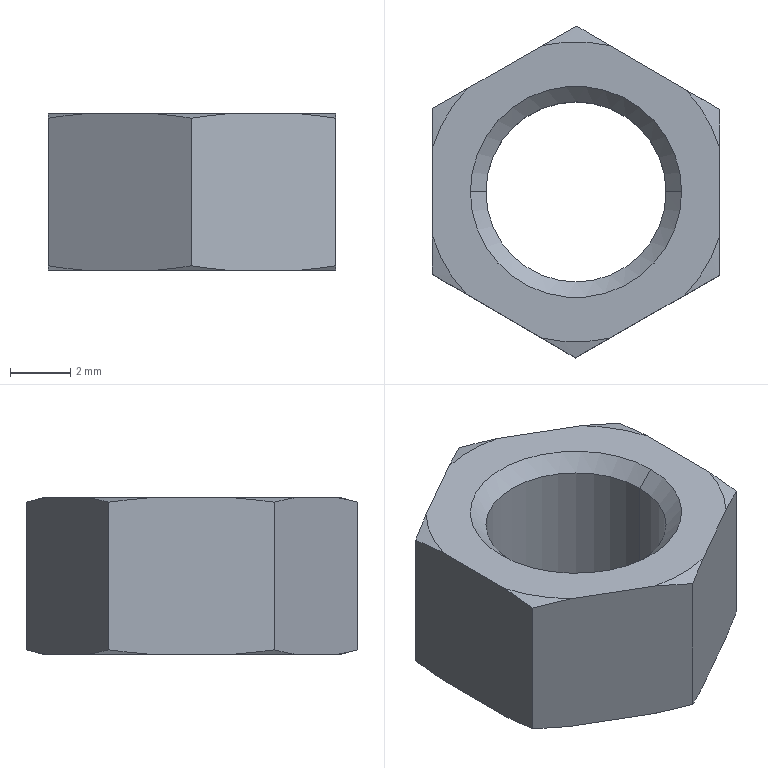Part | SolidWorks | features Cut 2, Chamfer 1, Extrusion 1 | 1 solid | 26 faces | box 9.591 x 11.05 x 5.2 mm | volume 259.734 mm3 | cone 16 | plane 8 | cylinder 2 | commonest cylinder face diameters 6 x2
STEP:
#1=CARTESIAN_POINT('',(-3.,0.,4.682));
#2=VERTEX_POINT('',#1);
#3=CARTESIAN_POINT('',(3.,0.,4.682));
#4=VERTEX_POINT('',#3);
#5=CARTESIAN_POINT('',(0.,0.,4.682));
#6=DIRECTION('',(0.,0.,1.));
#7=DIRECTION('',(-1.,0.,0.));
#8=AXIS2_PLACEMENT_3D('',#5,#6,#7);
#9=CIRCLE('',#8,3.);
#10=EDGE_CURVE('',#2,#4,#9,.T.);
#11=ORIENTED_EDGE('',*,*,#10,.F.);
#12=CARTESIAN_POINT('',(-3.518,0.,5.2));
#13=VERTEX_POINT('',#12);
#14=CARTESIAN_POINT('',(-3.,0.,4.682));
#15=DIRECTION('',(-0.7071,0.,0.7071));
#16=VECTOR('',#15,1000.);
#17=LINE('',#14,#16);
#18=EDGE_CURVE('',#2,#13,#17,.T.);
#19=ORIENTED_EDGE('',*,*,#18,.T.);
#20=CARTESIAN_POINT('',(3.518,0.,5.2));
#21=VERTEX_POINT('',#20);
#22=CARTESIAN_POINT('',(0.,0.,5.2));
#23=DIRECTION('',(0.,0.,-1.));
#24=DIRECTION('',(-1.,0.,0.));
#25=AXIS2_PLACEMENT_3D('',#22,#23,#24);
#26=CIRCLE('',#25,3.518);
#27=EDGE_CURVE('',#21,#13,#26,.T.);
#28=ORIENTED_EDGE('',*,*,#27,.F.);
#29=CARTESIAN_POINT('',(3.,0.,4.682));
#30=DIRECTION('',(0.7071,0.,0.7071));
#31=VECTOR('',#30,1000.);
#32=LINE('',#29,#31);
#33=EDGE_CURVE('',#4,#21,#32,.T.);
#34=ORIENTED_EDGE('',*,*,#33,.F.);
#35=EDGE_LOOP('',(#11,#19,#28,#34));
#36=FACE_OUTER_BOUND('',#35,.T.);
#37=CARTESIAN_POINT('',(0.,0.,4.682));
#38=DIRECTION('',(0.,0.,1.));
#39=DIRECTION('',(1.,0.,0.));
#40=AXIS2_PLACEMENT_3D('',#37,#38,#39);
#41=CONICAL_SURFACE('',#40,3.,0.7854);
#42=ADVANCED_FACE('',(#36),#41,.F.);
#43=CARTESIAN_POINT('',(3.,0.,0.5179));
#44=VERTEX_POINT('',#43);
#45=CARTESIAN_POINT('',(-3.,0.,0.5179));
#46=VERTEX_POINT('',#45);
#47=CARTESIAN_POINT('',(0.,0.,0.5179));
#48=DIRECTION('',(0.,0.,-1.));
#49=DIRECTION('',(-1.,0.,0.));
#50=AXIS2_PLACEMENT_3D('',#47,#48,#49);
#51=CIRCLE('',#50,3.);
#52=EDGE_CURVE('',#44,#46,#51,.T.);
#53=ORIENTED_EDGE('',*,*,#52,.F.);
#54=CARTESIAN_POINT('',(3.518,0.,0.));
#55=VERTEX_POINT('',#54);
#56=CARTESIAN_POINT('',(3.518,0.,0.));
#57=DIRECTION('',(0.7071,0.,-0.7071));
#58=VECTOR('',#57,1000.);
#59=LINE('',#56,#58);
#60=EDGE_CURVE('',#44,#55,#59,.T.);
#61=ORIENTED_EDGE('',*,*,#60,.T.);
#62=CARTESIAN_POINT('',(-3.518,0.,0.));
#63=VERTEX_POINT('',#62);
#64=CARTESIAN_POINT('',(0.,0.,0.));
#65=DIRECTION('',(0.,0.,1.));
#66=DIRECTION('',(-1.,0.,0.));
#67=AXIS2_PLACEMENT_3D('',#64,#65,#66);
#68=CIRCLE('',#67,3.518);
#69=EDGE_CURVE('',#63,#55,#68,.T.);
#70=ORIENTED_EDGE('',*,*,#69,.F.);
#71=CARTESIAN_POINT('',(-3.518,0.,0.));
#72=DIRECTION('',(-0.7071,0.,-0.7071));
#73=VECTOR('',#72,1000.);
#74=LINE('',#71,#73);
#75=EDGE_CURVE('',#46,#63,#74,.T.);
#76=ORIENTED_EDGE('',*,*,#75,.F.);
#77=EDGE_LOOP('',(#53,#61,#70,#76));
#78=FACE_OUTER_BOUND('',#77,.T.);
#79=CARTESIAN_POINT('',(0.,0.,0.));
#80=DIRECTION('',(0.,0.,-1.));
#81=DIRECTION('',(-1.,0.,0.));
#82=AXIS2_PLACEMENT_3D('',#79,#80,#81);
#83=CONICAL_SURFACE('',#82,3.518,0.7854);
#84=ADVANCED_FACE('',(#78),#83,.F.);
#85=ORIENTED_EDGE('',*,*,#10,.T.);
#86=CARTESIAN_POINT('',(3.,0.,5.2));
#87=DIRECTION('',(0.,0.,-1.));
#88=VECTOR('',#87,1000.);
#89=LINE('',#86,#88);
#90=EDGE_CURVE('',#4,#44,#89,.T.);
#91=ORIENTED_EDGE('',*,*,#90,.T.);
#92=ORIENTED_EDGE('',*,*,#52,.T.);
#93=CARTESIAN_POINT('',(-3.,0.,5.2));
#94=DIRECTION('',(0.,0.,-1.));
#95=VECTOR('',#94,1000.);
#96=LINE('',#93,#95);
#97=EDGE_CURVE('',#2,#46,#96,.T.);
#98=ORIENTED_EDGE('',*,*,#97,.F.);
#99=EDGE_LOOP('',(#85,#91,#92,#98));
#100=FACE_OUTER_BOUND('',#99,.T.);
#101=CARTESIAN_POINT('',(0.,0.,5.2));
#102=DIRECTION('',(0.,0.,-1.));
#103=DIRECTION('',(-1.,0.,0.));
#104=AXIS2_PLACEMENT_3D('',#101,#102,#103);
#105=CYLINDRICAL_SURFACE('',#104,3.);
#106=ADVANCED_FACE('',(#100),#105,.F.);
#107=CARTESIAN_POINT('',(4.796,2.744,5.059));
#108=VERTEX_POINT('',#107);
#109=CARTESIAN_POINT('',(3.663,3.404,5.2));
#110=VERTEX_POINT('',#109);
#111=CARTESIAN_POINT('',(4.796,2.744,5.059));
#112=CARTESIAN_POINT('',(4.419,2.963,5.118));
#113=CARTESIAN_POINT('',(4.042,3.183,5.166));
#114=CARTESIAN_POINT('',(3.663,3.404,5.2));
#115=B_SPLINE_CURVE_WITH_KNOTS('',3,(#111,#112,#113,#114),.UNSPECIFIED.,.F.,.F.,(4,4),(0.005302,0.006621),.UNSPECIFIED.);
#116=EDGE_CURVE('',#108,#110,#115,.T.);
#117=ORIENTED_EDGE('',*,*,#116,.F.);
#118=CARTESIAN_POINT('',(4.796,2.744,0.1407));
#119=VERTEX_POINT('',#118);
#120=CARTESIAN_POINT('',(4.796,2.744,5.2));
#121=DIRECTION('',(0.,0.,-1.));
#122=VECTOR('',#121,1000.);
#123=LINE('',#120,#122);
#124=EDGE_CURVE('',#108,#119,#123,.T.);
#125=ORIENTED_EDGE('',*,*,#124,.T.);
#126=CARTESIAN_POINT('',(3.663,3.404,0.));
#127=VERTEX_POINT('',#126);
#128=CARTESIAN_POINT('',(3.663,3.404,0.));
#129=CARTESIAN_POINT('',(4.042,3.183,0.03416));
#130=CARTESIAN_POINT('',(4.42,2.963,0.08238));
#131=CARTESIAN_POINT('',(4.796,2.744,0.1407));
#132=B_SPLINE_CURVE_WITH_KNOTS('',3,(#128,#129,#130,#131),.UNSPECIFIED.,.F.,.F.,(4,4),(0.009502,0.0108),.UNSPECIFIED.);
#133=EDGE_CURVE('',#127,#119,#132,.T.);
#134=ORIENTED_EDGE('',*,*,#133,.F.);
#135=CARTESIAN_POINT('',(1.155,4.865,0.));
#136=VERTEX_POINT('',#135);
#137=CARTESIAN_POINT('',(4.796,2.744,0.));
#138=DIRECTION('',(-0.8641,0.5034,0.));
#139=VECTOR('',#138,1000.);
#140=LINE('',#137,#139);
#141=EDGE_CURVE('',#127,#136,#140,.T.);
#142=ORIENTED_EDGE('',*,*,#141,.T.);
#143=CARTESIAN_POINT('',(0.02173,5.525,0.1407));
#144=VERTEX_POINT('',#143);
#145=CARTESIAN_POINT('',(0.02173,5.525,0.1407));
#146=CARTESIAN_POINT('',(0.3982,5.306,0.0823));
#147=CARTESIAN_POINT('',(0.7758,5.086,0.03411));
#148=CARTESIAN_POINT('',(1.155,4.865,0.));
#149=B_SPLINE_CURVE_WITH_KNOTS('',3,(#145,#146,#147,#148),.UNSPECIFIED.,.F.,.F.,(4,4),(0.005302,0.006621),.UNSPECIFIED.);
#150=EDGE_CURVE('',#144,#136,#149,.T.);
#151=ORIENTED_EDGE('',*,*,#150,.F.);
#152=CARTESIAN_POINT('',(0.02173,5.525,5.059));
#153=VERTEX_POINT('',#152);
#154=CARTESIAN_POINT('',(0.02173,5.525,5.2));
#155=DIRECTION('',(0.,0.,-1.));
#156=VECTOR('',#155,1000.);
#157=LINE('',#154,#156);
#158=EDGE_CURVE('',#153,#144,#157,.T.);
#159=ORIENTED_EDGE('',*,*,#158,.F.);
#160=CARTESIAN_POINT('',(1.155,4.865,5.2));
#161=VERTEX_POINT('',#160);
#162=CARTESIAN_POINT('',(1.155,4.865,5.2));
#163=CARTESIAN_POINT('',(0.7753,5.086,5.166));
#164=CARTESIAN_POINT('',(0.3977,5.306,5.118));
#165=CARTESIAN_POINT('',(0.02173,5.525,5.059));
#166=B_SPLINE_CURVE_WITH_KNOTS('',3,(#162,#163,#164,#165),.UNSPECIFIED.,.F.,.F.,(4,4),(0.009502,0.0108),.UNSPECIFIED.);
#167=EDGE_CURVE('',#161,#153,#166,.T.);
#168=ORIENTED_EDGE('',*,*,#167,.F.);
#169=CARTESIAN_POINT('',(4.796,2.744,5.2));
#170=DIRECTION('',(-0.8641,0.5034,0.));
#171=VECTOR('',#170,1000.);
#172=LINE('',#169,#171);
#173=EDGE_CURVE('',#110,#161,#172,.T.);
#174=ORIENTED_EDGE('',*,*,#173,.F.);
#175=EDGE_LOOP('',(#117,#125,#134,#142,#151,#159,#168,#174));
#176=FACE_OUTER_BOUND('',#175,.T.);
#177=CARTESIAN_POINT('',(4.796,2.744,5.2));
#178=DIRECTION('',(-0.5034,-0.8641,0.));
#179=DIRECTION('',(0.8641,-0.5034,0.));
#180=AXIS2_PLACEMENT_3D('',#177,#178,#179);
#181=PLANE('',#180);
#182=ADVANCED_FACE('',(#176),#181,.F.);
#183=CARTESIAN_POINT('',(-1.117,4.874,5.2));
#184=VERTEX_POINT('',#183);
#185=CARTESIAN_POINT('',(0.02173,5.525,5.059));
#186=CARTESIAN_POINT('',(-0.3565,5.309,5.118));
#187=CARTESIAN_POINT('',(-0.7358,5.092,5.166));
#188=CARTESIAN_POINT('',(-1.117,4.874,5.2));
#189=B_SPLINE_CURVE_WITH_KNOTS('',3,(#185,#186,#187,#188),.UNSPECIFIED.,.F.,.F.,(4,4),(0.005278,0.006597),.UNSPECIFIED.);
#190=EDGE_CURVE('',#153,#184,#189,.T.);
#191=ORIENTED_EDGE('',*,*,#190,.F.);
#192=ORIENTED_EDGE('',*,*,#158,.T.);
#193=CARTESIAN_POINT('',(-1.117,4.874,0.));
#194=VERTEX_POINT('',#193);
#195=CARTESIAN_POINT('',(-1.117,4.874,0.));
#196=CARTESIAN_POINT('',(-0.7353,5.092,0.03416));
#197=CARTESIAN_POINT('',(-0.3559,5.309,0.08238));
#198=CARTESIAN_POINT('',(0.02173,5.525,0.1407));
#199=B_SPLINE_CURVE_WITH_KNOTS('',3,(#195,#196,#197,#198),.UNSPECIFIED.,.F.,.F.,(4,4),(0.009478,0.01077),.UNSPECIFIED.);
#200=EDGE_CURVE('',#194,#144,#199,.T.);
#201=ORIENTED_EDGE('',*,*,#200,.F.);
#202=CARTESIAN_POINT('',(-3.636,3.433,0.));
#203=VERTEX_POINT('',#202);
#204=CARTESIAN_POINT('',(0.02173,5.525,0.));
#205=DIRECTION('',(-0.868,-0.4966,0.));
#206=VECTOR('',#205,1000.);
#207=LINE('',#204,#206);
#208=EDGE_CURVE('',#194,#203,#207,.T.);
#209=ORIENTED_EDGE('',*,*,#208,.T.);
#210=CARTESIAN_POINT('',(-4.774,2.781,0.1407));
#211=VERTEX_POINT('',#210);
#212=CARTESIAN_POINT('',(-4.774,2.781,0.1407));
#213=CARTESIAN_POINT('',(-4.396,2.998,0.0823));
#214=CARTESIAN_POINT('',(-4.016,3.215,0.03411));
#215=CARTESIAN_POINT('',(-3.636,3.433,0.));
#216=B_SPLINE_CURVE_WITH_KNOTS('',3,(#212,#213,#214,#215),.UNSPECIFIED.,.F.,.F.,(4,4),(0.005278,0.006597),.UNSPECIFIED.);
#217=EDGE_CURVE('',#211,#203,#216,.T.);
#218=ORIENTED_EDGE('',*,*,#217,.F.);
#219=CARTESIAN_POINT('',(-4.774,2.781,5.059));
#220=VERTEX_POINT('',#219);
#221=CARTESIAN_POINT('',(-4.774,2.781,5.2));
#222=DIRECTION('',(0.,0.,-1.));
#223=VECTOR('',#222,1000.);
#224=LINE('',#221,#223);
#225=EDGE_CURVE('',#220,#211,#224,.T.);
#226=ORIENTED_EDGE('',*,*,#225,.F.);
#227=CARTESIAN_POINT('',(-3.636,3.433,5.2));
#228=VERTEX_POINT('',#227);
#229=CARTESIAN_POINT('',(-3.636,3.433,5.2));
#230=CARTESIAN_POINT('',(-4.017,3.214,5.166));
#231=CARTESIAN_POINT('',(-4.396,2.997,5.118));
#232=CARTESIAN_POINT('',(-4.774,2.781,5.059));
#233=B_SPLINE_CURVE_WITH_KNOTS('',3,(#229,#230,#231,#232),.UNSPECIFIED.,.F.,.F.,(4,4),(0.009478,0.01077),.UNSPECIFIED.);
#234=EDGE_CURVE('',#228,#220,#233,.T.);
#235=ORIENTED_EDGE('',*,*,#234,.F.);
#236=CARTESIAN_POINT('',(0.02173,5.525,5.2));
#237=DIRECTION('',(-0.868,-0.4966,0.));
#238=VECTOR('',#237,1000.);
#239=LINE('',#236,#238);
#240=EDGE_CURVE('',#184,#228,#239,.T.);
#241=ORIENTED_EDGE('',*,*,#240,.F.);
#242=EDGE_LOOP('',(#191,#192,#201,#209,#218,#226,#235,#241));
#243=FACE_OUTER_BOUND('',#242,.T.);
#244=CARTESIAN_POINT('',(0.02173,5.525,5.2));
#245=DIRECTION('',(0.4966,-0.868,0.));
#246=DIRECTION('',(0.868,0.4966,0.));
#247=AXIS2_PLACEMENT_3D('',#244,#245,#246);
#248=PLANE('',#247);
#249=ADVANCED_FACE('',(#243),#248,.F.);
#250=CARTESIAN_POINT('',(-4.779,1.47,5.2));
#251=VERTEX_POINT('',#250);
#252=CARTESIAN_POINT('',(-4.774,2.781,5.059));
#253=CARTESIAN_POINT('',(-4.776,2.345,5.118));
#254=CARTESIAN_POINT('',(-4.777,1.908,5.166));
#255=CARTESIAN_POINT('',(-4.779,1.47,5.2));
#256=B_SPLINE_CURVE_WITH_KNOTS('',3,(#252,#253,#254,#255),.UNSPECIFIED.,.F.,.F.,(4,4),(0.004575,0.005894),.UNSPECIFIED.);
#257=EDGE_CURVE('',#220,#251,#256,.T.);
#258=ORIENTED_EDGE('',*,*,#257,.F.);
#259=ORIENTED_EDGE('',*,*,#225,.T.);
#260=CARTESIAN_POINT('',(-4.779,1.47,0.));
#261=VERTEX_POINT('',#260);
#262=CARTESIAN_POINT('',(-4.779,1.47,0.));
#263=CARTESIAN_POINT('',(-4.777,1.909,0.03411));
#264=CARTESIAN_POINT('',(-4.776,2.346,0.08237));
#265=CARTESIAN_POINT('',(-4.774,2.781,0.1407));
#266=B_SPLINE_CURVE_WITH_KNOTS('',3,(#262,#263,#264,#265),.UNSPECIFIED.,.F.,.F.,(4,4),(0.008778,0.01007),.UNSPECIFIED.);
#267=EDGE_CURVE('',#261,#211,#266,.T.);
#268=ORIENTED_EDGE('',*,*,#267,.F.);
#269=CARTESIAN_POINT('',(-4.79,-1.432,0.));
#270=VERTEX_POINT('',#269);
#271=CARTESIAN_POINT('',(-4.774,2.781,0.));
#272=DIRECTION('',(-0.003934,-1.,0.));
#273=VECTOR('',#272,1000.);
#274=LINE('',#271,#273);
#275=EDGE_CURVE('',#261,#270,#274,.T.);
#276=ORIENTED_EDGE('',*,*,#275,.T.);
#277=CARTESIAN_POINT('',(-4.796,-2.744,0.1407));
#278=VERTEX_POINT('',#277);
#279=CARTESIAN_POINT('',(-4.796,-2.744,0.1407));
#280=CARTESIAN_POINT('',(-4.794,-2.308,0.08228));
#281=CARTESIAN_POINT('',(-4.792,-1.871,0.0341));
#282=CARTESIAN_POINT('',(-4.79,-1.432,0.));
#283=B_SPLINE_CURVE_WITH_KNOTS('',3,(#279,#280,#281,#282),.UNSPECIFIED.,.F.,.F.,(4,4),(0.004575,0.005894),.UNSPECIFIED.);
#284=EDGE_CURVE('',#278,#270,#283,.T.);
#285=ORIENTED_EDGE('',*,*,#284,.F.);
#286=CARTESIAN_POINT('',(-4.796,-2.744,5.059));
#287=VERTEX_POINT('',#286);
#288=CARTESIAN_POINT('',(-4.796,-2.744,5.2));
#289=DIRECTION('',(0.,0.,-1.));
#290=VECTOR('',#289,1000.);
#291=LINE('',#288,#290);
#292=EDGE_CURVE('',#287,#278,#291,.T.);
#293=ORIENTED_EDGE('',*,*,#292,.F.);
#294=CARTESIAN_POINT('',(-4.79,-1.432,5.2));
#295=VERTEX_POINT('',#294);
#296=CARTESIAN_POINT('',(-4.79,-1.432,5.2));
#297=CARTESIAN_POINT('',(-4.792,-1.871,5.166));
#298=CARTESIAN_POINT('',(-4.794,-2.308,5.118));
#299=CARTESIAN_POINT('',(-4.796,-2.744,5.059));
#300=B_SPLINE_CURVE_WITH_KNOTS('',3,(#296,#297,#298,#299),.UNSPECIFIED.,.F.,.F.,(4,4),(0.008778,0.01007),.UNSPECIFIED.);
#301=EDGE_CURVE('',#295,#287,#300,.T.);
#302=ORIENTED_EDGE('',*,*,#301,.F.);
#303=CARTESIAN_POINT('',(-4.774,2.781,5.2));
#304=DIRECTION('',(-0.003934,-1.,0.));
#305=VECTOR('',#304,1000.);
#306=LINE('',#303,#305);
#307=EDGE_CURVE('',#251,#295,#306,.T.);
#308=ORIENTED_EDGE('',*,*,#307,.F.);
#309=EDGE_LOOP('',(#258,#259,#268,#276,#285,#293,#302,#308));
#310=FACE_OUTER_BOUND('',#309,.T.);
#311=CARTESIAN_POINT('',(-4.774,2.781,5.2));
#312=DIRECTION('',(1.,-0.003934,0.));
#313=DIRECTION('',(0.003934,1.,0.));
#314=AXIS2_PLACEMENT_3D('',#311,#312,#313);
#315=PLANE('',#314);
#316=ADVANCED_FACE('',(#310),#315,.F.);
#317=CARTESIAN_POINT('',(-3.663,-3.404,5.2));
#318=VERTEX_POINT('',#317);
#319=CARTESIAN_POINT('',(-4.796,-2.744,5.059));
#320=CARTESIAN_POINT('',(-4.419,-2.963,5.118));
#321=CARTESIAN_POINT('',(-4.042,-3.183,5.166));
#322=CARTESIAN_POINT('',(-3.663,-3.404,5.2));
#323=B_SPLINE_CURVE_WITH_KNOTS('',3,(#319,#320,#321,#322),.UNSPECIFIED.,.F.,.F.,(4,4),(0.005302,0.006621),.UNSPECIFIED.);
#324=EDGE_CURVE('',#287,#318,#323,.T.);
#325=ORIENTED_EDGE('',*,*,#324,.F.);
#326=ORIENTED_EDGE('',*,*,#292,.T.);
#327=CARTESIAN_POINT('',(-3.663,-3.404,0.));
#328=VERTEX_POINT('',#327);
#329=CARTESIAN_POINT('',(-3.663,-3.404,0.));
#330=CARTESIAN_POINT('',(-4.042,-3.183,0.03416));
#331=CARTESIAN_POINT('',(-4.42,-2.963,0.08238));
#332=CARTESIAN_POINT('',(-4.796,-2.744,0.1407));
#333=B_SPLINE_CURVE_WITH_KNOTS('',3,(#329,#330,#331,#332),.UNSPECIFIED.,.F.,.F.,(4,4),(0.009502,0.0108),.UNSPECIFIED.);
#334=EDGE_CURVE('',#328,#278,#333,.T.);
#335=ORIENTED_EDGE('',*,*,#334,.F.);
#336=CARTESIAN_POINT('',(-1.155,-4.865,0.));
#337=VERTEX_POINT('',#336);
#338=CARTESIAN_POINT('',(-4.796,-2.744,0.));
#339=DIRECTION('',(0.8641,-0.5034,0.));
#340=VECTOR('',#339,1000.);
#341=LINE('',#338,#340);
#342=EDGE_CURVE('',#328,#337,#341,.T.);
#343=ORIENTED_EDGE('',*,*,#342,.T.);
#344=CARTESIAN_POINT('',(-0.02173,-5.525,0.1407));
#345=VERTEX_POINT('',#344);
#346=CARTESIAN_POINT('',(-0.02173,-5.525,0.1407));
#347=CARTESIAN_POINT('',(-0.3982,-5.306,0.0823));
#348=CARTESIAN_POINT('',(-0.7758,-5.086,0.03411));
#349=CARTESIAN_POINT('',(-1.155,-4.865,0.));
#350=B_SPLINE_CURVE_WITH_KNOTS('',3,(#346,#347,#348,#349),.UNSPECIFIED.,.F.,.F.,(4,4),(0.005302,0.006621),.UNSPECIFIED.);
#351=EDGE_CURVE('',#345,#337,#350,.T.);
#352=ORIENTED_EDGE('',*,*,#351,.F.);
#353=CARTESIAN_POINT('',(-0.02173,-5.525,5.059));
#354=VERTEX_POINT('',#353);
#355=CARTESIAN_POINT('',(-0.02173,-5.525,5.2));
#356=DIRECTION('',(0.,0.,-1.));
#357=VECTOR('',#356,1000.);
#358=LINE('',#355,#357);
#359=EDGE_CURVE('',#354,#345,#358,.T.);
#360=ORIENTED_EDGE('',*,*,#359,.F.);
#361=CARTESIAN_POINT('',(-1.155,-4.865,5.2));
#362=VERTEX_POINT('',#361);
#363=CARTESIAN_POINT('',(-1.155,-4.865,5.2));
#364=CARTESIAN_POINT('',(-0.7753,-5.086,5.166));
#365=CARTESIAN_POINT('',(-0.3977,-5.306,5.118));
#366=CARTESIAN_POINT('',(-0.02173,-5.525,5.059));
#367=B_SPLINE_CURVE_WITH_KNOTS('',3,(#363,#364,#365,#366),.UNSPECIFIED.,.F.,.F.,(4,4),(0.009502,0.0108),.UNSPECIFIED.);
#368=EDGE_CURVE('',#362,#354,#367,.T.);
#369=ORIENTED_EDGE('',*,*,#368,.F.);
#370=CARTESIAN_POINT('',(-4.796,-2.744,5.2));
#371=DIRECTION('',(0.8641,-0.5034,0.));
#372=VECTOR('',#371,1000.);
#373=LINE('',#370,#372);
#374=EDGE_CURVE('',#318,#362,#373,.T.);
#375=ORIENTED_EDGE('',*,*,#374,.F.);
#376=EDGE_LOOP('',(#325,#326,#335,#343,#352,#360,#369,#375));
#377=FACE_OUTER_BOUND('',#376,.T.);
#378=CARTESIAN_POINT('',(-4.796,-2.744,5.2));
#379=DIRECTION('',(0.5034,0.8641,0.));
#380=DIRECTION('',(-0.8641,0.5034,0.));
#381=AXIS2_PLACEMENT_3D('',#378,#379,#380);
#382=PLANE('',#381);
#383=ADVANCED_FACE('',(#377),#382,.F.);
#384=CARTESIAN_POINT('',(1.117,-4.874,5.2));
#385=VERTEX_POINT('',#384);
#386=CARTESIAN_POINT('',(-0.02173,-5.525,5.059));
#387=CARTESIAN_POINT('',(0.3565,-5.309,5.118));
#388=CARTESIAN_POINT('',(0.7358,-5.092,5.166));
#389=CARTESIAN_POINT('',(1.117,-4.874,5.2));
#390=B_SPLINE_CURVE_WITH_KNOTS('',3,(#386,#387,#388,#389),.UNSPECIFIED.,.F.,.F.,(4,4),(0.005278,0.006597),.UNSPECIFIED.);
#391=EDGE_CURVE('',#354,#385,#390,.T.);
#392=ORIENTED_EDGE('',*,*,#391,.F.);
#393=ORIENTED_EDGE('',*,*,#359,.T.);
#394=CARTESIAN_POINT('',(1.117,-4.874,0.));
#395=VERTEX_POINT('',#394);
#396=CARTESIAN_POINT('',(1.117,-4.874,0.));
#397=CARTESIAN_POINT('',(0.7353,-5.092,0.03416));
#398=CARTESIAN_POINT('',(0.3559,-5.309,0.08238));
#399=CARTESIAN_POINT('',(-0.02173,-5.525,0.1407));
#400=B_SPLINE_CURVE_WITH_KNOTS('',3,(#396,#397,#398,#399),.UNSPECIFIED.,.F.,.F.,(4,4),(0.009478,0.01077),.UNSPECIFIED.);
#401=EDGE_CURVE('',#395,#345,#400,.T.);
#402=ORIENTED_EDGE('',*,*,#401,.F.);
#403=CARTESIAN_POINT('',(3.636,-3.433,0.));
#404=VERTEX_POINT('',#403);
#405=CARTESIAN_POINT('',(-0.02173,-5.525,0.));
#406=DIRECTION('',(0.868,0.4966,0.));
#407=VECTOR('',#406,1000.);
#408=LINE('',#405,#407);
#409=EDGE_CURVE('',#395,#404,#408,.T.);
#410=ORIENTED_EDGE('',*,*,#409,.T.);
#411=CARTESIAN_POINT('',(4.774,-2.781,0.1407));
#412=VERTEX_POINT('',#411);
#413=CARTESIAN_POINT('',(4.774,-2.781,0.1407));
#414=CARTESIAN_POINT('',(4.396,-2.998,0.0823));
#415=CARTESIAN_POINT('',(4.016,-3.215,0.03411));
#416=CARTESIAN_POINT('',(3.636,-3.433,0.));
#417=B_SPLINE_CURVE_WITH_KNOTS('',3,(#413,#414,#415,#416),.UNSPECIFIED.,.F.,.F.,(4,4),(0.005278,0.006597),.UNSPECIFIED.);
#418=EDGE_CURVE('',#412,#404,#417,.T.);
#419=ORIENTED_EDGE('',*,*,#418,.F.);
#420=CARTESIAN_POINT('',(4.774,-2.781,5.059));
#421=VERTEX_POINT('',#420);
#422=CARTESIAN_POINT('',(4.774,-2.781,5.2));
#423=DIRECTION('',(0.,0.,-1.));
#424=VECTOR('',#423,1000.);
#425=LINE('',#422,#424);
#426=EDGE_CURVE('',#421,#412,#425,.T.);
#427=ORIENTED_EDGE('',*,*,#426,.F.);
#428=CARTESIAN_POINT('',(3.636,-3.433,5.2));
#429=VERTEX_POINT('',#428);
#430=CARTESIAN_POINT('',(3.636,-3.433,5.2));
#431=CARTESIAN_POINT('',(4.017,-3.214,5.166));
#432=CARTESIAN_POINT('',(4.396,-2.997,5.118));
#433=CARTESIAN_POINT('',(4.774,-2.781,5.059));
#434=B_SPLINE_CURVE_WITH_KNOTS('',3,(#430,#431,#432,#433),.UNSPECIFIED.,.F.,.F.,(4,4),(0.009478,0.01077),.UNSPECIFIED.);
#435=EDGE_CURVE('',#429,#421,#434,.T.);
#436=ORIENTED_EDGE('',*,*,#435,.F.);
#437=CARTESIAN_POINT('',(-0.02173,-5.525,5.2));
#438=DIRECTION('',(0.868,0.4966,0.));
#439=VECTOR('',#438,1000.);
#440=LINE('',#437,#439);
#441=EDGE_CURVE('',#385,#429,#440,.T.);
#442=ORIENTED_EDGE('',*,*,#441,.F.);
#443=EDGE_LOOP('',(#392,#393,#402,#410,#419,#427,#436,#442));
#444=FACE_OUTER_BOUND('',#443,.T.);
#445=CARTESIAN_POINT('',(-0.02173,-5.525,5.2));
#446=DIRECTION('',(-0.4966,0.868,0.));
#447=DIRECTION('',(-0.868,-0.4966,0.));
#448=AXIS2_PLACEMENT_3D('',#445,#446,#447);
#449=PLANE('',#448);
#450=ADVANCED_FACE('',(#444),#449,.F.);
#451=CARTESIAN_POINT('',(4.779,-1.47,5.2));
#452=VERTEX_POINT('',#451);
#453=CARTESIAN_POINT('',(4.774,-2.781,5.059));
#454=CARTESIAN_POINT('',(4.776,-2.345,5.118));
#455=CARTESIAN_POINT('',(4.777,-1.908,5.166));
#456=CARTESIAN_POINT('',(4.779,-1.47,5.2));
#457=B_SPLINE_CURVE_WITH_KNOTS('',3,(#453,#454,#455,#456),.UNSPECIFIED.,.F.,.F.,(4,4),(0.004575,0.005894),.UNSPECIFIED.);
#458=EDGE_CURVE('',#421,#452,#457,.T.);
#459=ORIENTED_EDGE('',*,*,#458,.F.);
#460=ORIENTED_EDGE('',*,*,#426,.T.);
#461=CARTESIAN_POINT('',(4.779,-1.47,0.));
#462=VERTEX_POINT('',#461);
#463=CARTESIAN_POINT('',(4.779,-1.47,0.));
#464=CARTESIAN_POINT('',(4.777,-1.909,0.03411));
#465=CARTESIAN_POINT('',(4.776,-2.346,0.08237));
#466=CARTESIAN_POINT('',(4.774,-2.781,0.1407));
#467=B_SPLINE_CURVE_WITH_KNOTS('',3,(#463,#464,#465,#466),.UNSPECIFIED.,.F.,.F.,(4,4),(0.008778,0.01007),.UNSPECIFIED.);
#468=EDGE_CURVE('',#462,#412,#467,.T.);
#469=ORIENTED_EDGE('',*,*,#468,.F.);
#470=CARTESIAN_POINT('',(4.79,1.432,0.));
#471=VERTEX_POINT('',#470);
#472=CARTESIAN_POINT('',(4.774,-2.781,0.));
#473=DIRECTION('',(0.003934,1.,0.));
#474=VECTOR('',#473,1000.);
#475=LINE('',#472,#474);
#476=EDGE_CURVE('',#462,#471,#475,.T.);
#477=ORIENTED_EDGE('',*,*,#476,.T.);
#478=CARTESIAN_POINT('',(4.796,2.744,0.1407));
#479=CARTESIAN_POINT('',(4.794,2.308,0.08228));
#480=CARTESIAN_POINT('',(4.792,1.871,0.0341));
#481=CARTESIAN_POINT('',(4.79,1.432,0.));
#482=B_SPLINE_CURVE_WITH_KNOTS('',3,(#478,#479,#480,#481),.UNSPECIFIED.,.F.,.F.,(4,4),(0.004575,0.005894),.UNSPECIFIED.);
#483=EDGE_CURVE('',#119,#471,#482,.T.);
#484=ORIENTED_EDGE('',*,*,#483,.F.);
#485=ORIENTED_EDGE('',*,*,#124,.F.);
#486=CARTESIAN_POINT('',(4.79,1.432,5.2));
#487=VERTEX_POINT('',#486);
#488=CARTESIAN_POINT('',(4.79,1.432,5.2));
#489=CARTESIAN_POINT('',(4.792,1.871,5.166));
#490=CARTESIAN_POINT('',(4.794,2.308,5.118));
#491=CARTESIAN_POINT('',(4.796,2.744,5.059));
#492=B_SPLINE_CURVE_WITH_KNOTS('',3,(#488,#489,#490,#491),.UNSPECIFIED.,.F.,.F.,(4,4),(0.008778,0.01007),.UNSPECIFIED.);
#493=EDGE_CURVE('',#487,#108,#492,.T.);
#494=ORIENTED_EDGE('',*,*,#493,.F.);
#495=CARTESIAN_POINT('',(4.774,-2.781,5.2));
#496=DIRECTION('',(0.003934,1.,0.));
#497=VECTOR('',#496,1000.);
#498=LINE('',#495,#497);
#499=EDGE_CURVE('',#452,#487,#498,.T.);
#500=ORIENTED_EDGE('',*,*,#499,.F.);
#501=EDGE_LOOP('',(#459,#460,#469,#477,#484,#485,#494,#500));
#502=FACE_OUTER_BOUND('',#501,.T.);
#503=CARTESIAN_POINT('',(4.774,-2.781,5.2));
#504=DIRECTION('',(-1.,0.003934,0.));
#505=DIRECTION('',(-0.003934,-1.,0.));
#506=AXIS2_PLACEMENT_3D('',#503,#504,#505);
#507=PLANE('',#506);
#508=ADVANCED_FACE('',(#502),#507,.F.);
#509=ORIENTED_EDGE('',*,*,#27,.T.);
#510=CARTESIAN_POINT('',(0.,0.,5.2));
#511=DIRECTION('',(0.,0.,-1.));
#512=DIRECTION('',(-1.,0.,0.));
#513=AXIS2_PLACEMENT_3D('',#510,#511,#512);
#514=CIRCLE('',#513,3.518);
#515=EDGE_CURVE('',#13,#21,#514,.T.);
#516=ORIENTED_EDGE('',*,*,#515,.T.);
#517=EDGE_LOOP('',(#509,#516));
#518=FACE_BOUND('',#517,.T.);
#519=CARTESIAN_POINT('',(0.,0.,5.2));
#520=DIRECTION('',(0.,0.,-1.));
#521=DIRECTION('',(-1.,0.,0.));
#522=AXIS2_PLACEMENT_3D('',#519,#520,#521);
#523=CIRCLE('',#522,5.);
#524=EDGE_CURVE('',#251,#228,#523,.T.);
#525=ORIENTED_EDGE('',*,*,#524,.F.);
#526=ORIENTED_EDGE('',*,*,#307,.T.);
#527=CARTESIAN_POINT('',(0.,0.,5.2));
#528=DIRECTION('',(0.,0.,-1.));
#529=DIRECTION('',(-1.,0.,0.));
#530=AXIS2_PLACEMENT_3D('',#527,#528,#529);
#531=CIRCLE('',#530,5.);
#532=EDGE_CURVE('',#318,#295,#531,.T.);
#533=ORIENTED_EDGE('',*,*,#532,.F.);
#534=ORIENTED_EDGE('',*,*,#374,.T.);
#535=CARTESIAN_POINT('',(0.,0.,5.2));
#536=DIRECTION('',(0.,0.,-1.));
#537=DIRECTION('',(-1.,0.,0.));
#538=AXIS2_PLACEMENT_3D('',#535,#536,#537);
#539=CIRCLE('',#538,5.);
#540=EDGE_CURVE('',#385,#362,#539,.T.);
#541=ORIENTED_EDGE('',*,*,#540,.F.);
#542=ORIENTED_EDGE('',*,*,#441,.T.);
#543=CARTESIAN_POINT('',(0.,0.,5.2));
#544=DIRECTION('',(0.,0.,-1.));
#545=DIRECTION('',(-1.,0.,0.));
#546=AXIS2_PLACEMENT_3D('',#543,#544,#545);
#547=CIRCLE('',#546,5.);
#548=EDGE_CURVE('',#452,#429,#547,.T.);
#549=ORIENTED_EDGE('',*,*,#548,.F.);
#550=ORIENTED_EDGE('',*,*,#499,.T.);
#551=CARTESIAN_POINT('',(0.,0.,5.2));
#552=DIRECTION('',(0.,0.,1.));
#553=DIRECTION('',(1.,0.,0.));
#554=AXIS2_PLACEMENT_3D('',#551,#552,#553);
#555=CIRCLE('',#554,5.);
#556=EDGE_CURVE('',#487,#110,#555,.T.);
#557=ORIENTED_EDGE('',*,*,#556,.T.);
#558=ORIENTED_EDGE('',*,*,#173,.T.);
#559=CARTESIAN_POINT('',(0.,0.,5.2));
#560=DIRECTION('',(0.,0.,-1.));
#561=DIRECTION('',(-1.,0.,0.));
#562=AXIS2_PLACEMENT_3D('',#559,#560,#561);
#563=CIRCLE('',#562,5.);
#564=EDGE_CURVE('',#184,#161,#563,.T.);
#565=ORIENTED_EDGE('',*,*,#564,.F.);
#566=ORIENTED_EDGE('',*,*,#240,.T.);
#567=EDGE_LOOP('',(#525,#526,#533,#534,#541,#542,#549,#550,#557,#558,#565,#566));
#568=FACE_OUTER_BOUND('',#567,.T.);
#569=CARTESIAN_POINT('',(9.57,-0.03764,5.2));
#570=DIRECTION('',(0.,0.,-1.));
#571=DIRECTION('',(-1.,0.,0.));
#572=AXIS2_PLACEMENT_3D('',#569,#570,#571);
#573=PLANE('',#572);
#574=ADVANCED_FACE('',(#518,#568),#573,.F.);
#575=ORIENTED_EDGE('',*,*,#69,.T.);
#576=CARTESIAN_POINT('',(0.,0.,0.));
#577=DIRECTION('',(0.,0.,1.));
#578=DIRECTION('',(-1.,0.,0.));
#579=AXIS2_PLACEMENT_3D('',#576,#577,#578);
#580=CIRCLE('',#579,3.518);
#581=EDGE_CURVE('',#55,#63,#580,.T.);
#582=ORIENTED_EDGE('',*,*,#581,.T.);
#583=EDGE_LOOP('',(#575,#582));
#584=FACE_BOUND('',#583,.T.);
#585=ORIENTED_EDGE('',*,*,#275,.F.);
#586=CARTESIAN_POINT('',(0.,0.,0.));
#587=DIRECTION('',(0.,0.,-1.));
#588=DIRECTION('',(-1.,0.,0.));
#589=AXIS2_PLACEMENT_3D('',#586,#587,#588);
#590=CIRCLE('',#589,5.);
#591=EDGE_CURVE('',#261,#203,#590,.T.);
#592=ORIENTED_EDGE('',*,*,#591,.T.);
#593=ORIENTED_EDGE('',*,*,#208,.F.);
#594=CARTESIAN_POINT('',(0.,0.,0.));
#595=DIRECTION('',(0.,0.,-1.));
#596=DIRECTION('',(-1.,0.,0.));
#597=AXIS2_PLACEMENT_3D('',#594,#595,#596);
#598=CIRCLE('',#597,5.);
#599=EDGE_CURVE('',#194,#136,#598,.T.);
#600=ORIENTED_EDGE('',*,*,#599,.T.);
#601=ORIENTED_EDGE('',*,*,#141,.F.);
#602=CARTESIAN_POINT('',(0.,0.,0.));
#603=DIRECTION('',(0.,0.,-1.));
#604=DIRECTION('',(-1.,0.,0.));
#605=AXIS2_PLACEMENT_3D('',#602,#603,#604);
#606=CIRCLE('',#605,5.);
#607=EDGE_CURVE('',#127,#471,#606,.T.);
#608=ORIENTED_EDGE('',*,*,#607,.T.);
#609=ORIENTED_EDGE('',*,*,#476,.F.);
#610=CARTESIAN_POINT('',(0.,0.,0.));
#611=DIRECTION('',(0.,0.,-1.));
#612=DIRECTION('',(-1.,0.,0.));
#613=AXIS2_PLACEMENT_3D('',#610,#611,#612);
#614=CIRCLE('',#613,5.);
#615=EDGE_CURVE('',#462,#404,#614,.T.);
#616=ORIENTED_EDGE('',*,*,#615,.T.);
#617=ORIENTED_EDGE('',*,*,#409,.F.);
#618=CARTESIAN_POINT('',(0.,0.,0.));
#619=DIRECTION('',(0.,0.,-1.));
#620=DIRECTION('',(-1.,0.,0.));
#621=AXIS2_PLACEMENT_3D('',#618,#619,#620);
#622=CIRCLE('',#621,5.);
#623=EDGE_CURVE('',#395,#337,#622,.T.);
#624=ORIENTED_EDGE('',*,*,#623,.T.);
#625=ORIENTED_EDGE('',*,*,#342,.F.);
#626=CARTESIAN_POINT('',(0.,0.,0.));
#627=DIRECTION('',(0.,0.,-1.));
#628=DIRECTION('',(-1.,0.,0.));
#629=AXIS2_PLACEMENT_3D('',#626,#627,#628);
#630=CIRCLE('',#629,5.);
#631=EDGE_CURVE('',#328,#270,#630,.T.);
#632=ORIENTED_EDGE('',*,*,#631,.T.);
#633=EDGE_LOOP('',(#585,#592,#593,#600,#601,#608,#609,#616,#617,#624,#625,#632));
#634=FACE_OUTER_BOUND('',#633,.T.);
#635=CARTESIAN_POINT('',(9.57,-0.03764,0.));
#636=DIRECTION('',(0.,0.,-1.));
#637=DIRECTION('',(-1.,0.,0.));
#638=AXIS2_PLACEMENT_3D('',#635,#636,#637);
#639=PLANE('',#638);
#640=ADVANCED_FACE('',(#584,#634),#639,.T.);
#641=ORIENTED_EDGE('',*,*,#90,.F.);
#642=CARTESIAN_POINT('',(0.,0.,4.682));
#643=DIRECTION('',(0.,0.,1.));
#644=DIRECTION('',(-1.,0.,0.));
#645=AXIS2_PLACEMENT_3D('',#642,#643,#644);
#646=CIRCLE('',#645,3.);
#647=EDGE_CURVE('',#4,#2,#646,.T.);
#648=ORIENTED_EDGE('',*,*,#647,.T.);
#649=ORIENTED_EDGE('',*,*,#97,.T.);
#650=CARTESIAN_POINT('',(0.,0.,0.5179));
#651=DIRECTION('',(0.,0.,-1.));
#652=DIRECTION('',(-1.,0.,0.));
#653=AXIS2_PLACEMENT_3D('',#650,#651,#652);
#654=CIRCLE('',#653,3.);
#655=EDGE_CURVE('',#46,#44,#654,.T.);
#656=ORIENTED_EDGE('',*,*,#655,.T.);
#657=EDGE_LOOP('',(#641,#648,#649,#656));
#658=FACE_OUTER_BOUND('',#657,.T.);
#659=CARTESIAN_POINT('',(0.,0.,5.2));
#660=DIRECTION('',(0.,0.,-1.));
#661=DIRECTION('',(-1.,0.,0.));
#662=AXIS2_PLACEMENT_3D('',#659,#660,#661);
#663=CYLINDRICAL_SURFACE('',#662,3.);
#664=ADVANCED_FACE('',(#658),#663,.F.);
#665=ORIENTED_EDGE('',*,*,#418,.T.);
#666=ORIENTED_EDGE('',*,*,#615,.F.);
#667=ORIENTED_EDGE('',*,*,#468,.T.);
#668=EDGE_LOOP('',(#665,#666,#667));
#669=FACE_OUTER_BOUND('',#668,.T.);
#670=CARTESIAN_POINT('',(0.,0.,0.));
#671=DIRECTION('',(0.,0.,1.));
#672=DIRECTION('',(-1.,0.,0.));
#673=AXIS2_PLACEMENT_3D('',#670,#671,#672);
#674=CONICAL_SURFACE('',#673,5.,1.309);
#675=ADVANCED_FACE('',(#669),#674,.T.);
#676=ORIENTED_EDGE('',*,*,#133,.T.);
#677=ORIENTED_EDGE('',*,*,#483,.T.);
#678=ORIENTED_EDGE('',*,*,#607,.F.);
#679=EDGE_LOOP('',(#676,#677,#678));
#680=FACE_OUTER_BOUND('',#679,.T.);
#681=CARTESIAN_POINT('',(0.,0.,0.));
#682=DIRECTION('',(0.,0.,1.));
#683=DIRECTION('',(-1.,0.,0.));
#684=AXIS2_PLACEMENT_3D('',#681,#682,#683);
#685=CONICAL_SURFACE('',#684,5.,1.309);
#686=ADVANCED_FACE('',(#680),#685,.T.);
#687=ORIENTED_EDGE('',*,*,#351,.T.);
#688=ORIENTED_EDGE('',*,*,#623,.F.);
#689=ORIENTED_EDGE('',*,*,#401,.T.);
#690=EDGE_LOOP('',(#687,#688,#689));
#691=FACE_OUTER_BOUND('',#690,.T.);
#692=CARTESIAN_POINT('',(0.,0.,0.));
#693=DIRECTION('',(0.,0.,1.));
#694=DIRECTION('',(-1.,0.,0.));
#695=AXIS2_PLACEMENT_3D('',#692,#693,#694);
#696=CONICAL_SURFACE('',#695,5.,1.309);
#697=ADVANCED_FACE('',(#691),#696,.T.);
#698=ORIENTED_EDGE('',*,*,#284,.T.);
#699=ORIENTED_EDGE('',*,*,#631,.F.);
#700=ORIENTED_EDGE('',*,*,#334,.T.);
#701=EDGE_LOOP('',(#698,#699,#700));
#702=FACE_OUTER_BOUND('',#701,.T.);
#703=CARTESIAN_POINT('',(0.,0.,0.));
#704=DIRECTION('',(0.,0.,1.));
#705=DIRECTION('',(-1.,0.,0.));
#706=AXIS2_PLACEMENT_3D('',#703,#704,#705);
#707=CONICAL_SURFACE('',#706,5.,1.309);
#708=ADVANCED_FACE('',(#702),#707,.T.);
#709=ORIENTED_EDGE('',*,*,#217,.T.);
#710=ORIENTED_EDGE('',*,*,#591,.F.);
#711=ORIENTED_EDGE('',*,*,#267,.T.);
#712=EDGE_LOOP('',(#709,#710,#711));
#713=FACE_OUTER_BOUND('',#712,.T.);
#714=CARTESIAN_POINT('',(0.,0.,0.));
#715=DIRECTION('',(0.,0.,1.));
#716=DIRECTION('',(-1.,0.,0.));
#717=AXIS2_PLACEMENT_3D('',#714,#715,#716);
#718=CONICAL_SURFACE('',#717,5.,1.309);
#719=ADVANCED_FACE('',(#713),#718,.T.);
#720=ORIENTED_EDGE('',*,*,#150,.T.);
#721=ORIENTED_EDGE('',*,*,#599,.F.);
#722=ORIENTED_EDGE('',*,*,#200,.T.);
#723=EDGE_LOOP('',(#720,#721,#722));
#724=FACE_OUTER_BOUND('',#723,.T.);
#725=CARTESIAN_POINT('',(0.,0.,0.));
#726=DIRECTION('',(0.,0.,1.));
#727=DIRECTION('',(-1.,0.,0.));
#728=AXIS2_PLACEMENT_3D('',#725,#726,#727);
#729=CONICAL_SURFACE('',#728,5.,1.309);
#730=ADVANCED_FACE('',(#724),#729,.T.);
#731=ORIENTED_EDGE('',*,*,#301,.T.);
#732=ORIENTED_EDGE('',*,*,#324,.T.);
#733=ORIENTED_EDGE('',*,*,#532,.T.);
#734=EDGE_LOOP('',(#731,#732,#733));
#735=FACE_OUTER_BOUND('',#734,.T.);
#736=CARTESIAN_POINT('',(0.,0.,5.2));
#737=DIRECTION('',(0.,0.,-1.));
#738=DIRECTION('',(1.,0.,0.));
#739=AXIS2_PLACEMENT_3D('',#736,#737,#738);
#740=CONICAL_SURFACE('',#739,5.,1.309);
#741=ADVANCED_FACE('',(#735),#740,.T.);
#742=ORIENTED_EDGE('',*,*,#368,.T.);
#743=ORIENTED_EDGE('',*,*,#391,.T.);
#744=ORIENTED_EDGE('',*,*,#540,.T.);
#745=EDGE_LOOP('',(#742,#743,#744));
#746=FACE_OUTER_BOUND('',#745,.T.);
#747=CARTESIAN_POINT('',(0.,0.,5.2));
#748=DIRECTION('',(0.,0.,-1.));
#749=DIRECTION('',(1.,0.,0.));
#750=AXIS2_PLACEMENT_3D('',#747,#748,#749);
#751=CONICAL_SURFACE('',#750,5.,1.309);
#752=ADVANCED_FACE('',(#746),#751,.T.);
#753=ORIENTED_EDGE('',*,*,#435,.T.);
#754=ORIENTED_EDGE('',*,*,#458,.T.);
#755=ORIENTED_EDGE('',*,*,#548,.T.);
#756=EDGE_LOOP('',(#753,#754,#755));
#757=FACE_OUTER_BOUND('',#756,.T.);
#758=CARTESIAN_POINT('',(0.,0.,5.2));
#759=DIRECTION('',(0.,0.,-1.));
#760=DIRECTION('',(1.,0.,0.));
#761=AXIS2_PLACEMENT_3D('',#758,#759,#760);
#762=CONICAL_SURFACE('',#761,5.,1.309);
#763=ADVANCED_FACE('',(#757),#762,.T.);
#764=ORIENTED_EDGE('',*,*,#116,.T.);
#765=ORIENTED_EDGE('',*,*,#556,.F.);
#766=ORIENTED_EDGE('',*,*,#493,.T.);
#767=EDGE_LOOP('',(#764,#765,#766));
#768=FACE_OUTER_BOUND('',#767,.T.);
#769=CARTESIAN_POINT('',(0.,0.,5.2));
#770=DIRECTION('',(0.,0.,-1.));
#771=DIRECTION('',(1.,0.,0.));
#772=AXIS2_PLACEMENT_3D('',#769,#770,#771);
#773=CONICAL_SURFACE('',#772,5.,1.309);
#774=ADVANCED_FACE('',(#768),#773,.T.);
#775=ORIENTED_EDGE('',*,*,#167,.T.);
#776=ORIENTED_EDGE('',*,*,#190,.T.);
#777=ORIENTED_EDGE('',*,*,#564,.T.);
#778=EDGE_LOOP('',(#775,#776,#777));
#779=FACE_OUTER_BOUND('',#778,.T.);
#780=CARTESIAN_POINT('',(0.,0.,5.2));
#781=DIRECTION('',(0.,0.,-1.));
#782=DIRECTION('',(1.,0.,0.));
#783=AXIS2_PLACEMENT_3D('',#780,#781,#782);
#784=CONICAL_SURFACE('',#783,5.,1.309);
#785=ADVANCED_FACE('',(#779),#784,.T.);
#786=ORIENTED_EDGE('',*,*,#234,.T.);
#787=ORIENTED_EDGE('',*,*,#257,.T.);
#788=ORIENTED_EDGE('',*,*,#524,.T.);
#789=EDGE_LOOP('',(#786,#787,#788));
#790=FACE_OUTER_BOUND('',#789,.T.);
#791=CARTESIAN_POINT('',(0.,0.,5.2));
#792=DIRECTION('',(0.,0.,-1.));
#793=DIRECTION('',(1.,0.,0.));
#794=AXIS2_PLACEMENT_3D('',#791,#792,#793);
#795=CONICAL_SURFACE('',#794,5.,1.309);
#796=ADVANCED_FACE('',(#790),#795,.T.);
#797=ORIENTED_EDGE('',*,*,#60,.F.);
#798=ORIENTED_EDGE('',*,*,#655,.F.);
#799=ORIENTED_EDGE('',*,*,#75,.T.);
#800=ORIENTED_EDGE('',*,*,#581,.F.);
#801=EDGE_LOOP('',(#797,#798,#799,#800));
#802=FACE_OUTER_BOUND('',#801,.T.);
#803=CARTESIAN_POINT('',(0.,0.,0.));
#804=DIRECTION('',(0.,0.,-1.));
#805=DIRECTION('',(-1.,0.,0.));
#806=AXIS2_PLACEMENT_3D('',#803,#804,#805);
#807=CONICAL_SURFACE('',#806,3.518,0.7854);
#808=ADVANCED_FACE('',(#802),#807,.F.);
#809=ORIENTED_EDGE('',*,*,#18,.F.);
#810=ORIENTED_EDGE('',*,*,#647,.F.);
#811=ORIENTED_EDGE('',*,*,#33,.T.);
#812=ORIENTED_EDGE('',*,*,#515,.F.);
#813=EDGE_LOOP('',(#809,#810,#811,#812));
#814=FACE_OUTER_BOUND('',#813,.T.);
#815=CARTESIAN_POINT('',(0.,0.,4.682));
#816=DIRECTION('',(0.,0.,1.));
#817=DIRECTION('',(1.,0.,0.));
#818=AXIS2_PLACEMENT_3D('',#815,#816,#817);
#819=CONICAL_SURFACE('',#818,3.,0.7854);
#820=ADVANCED_FACE('',(#814),#819,.F.);
#821=CLOSED_SHELL('',(#42,#84,#106,#182,#249,#316,#383,#450,#508,#574,#640,#664,#675,#686,#697,#708,#719,#730,#741,#752,#763,#774,#785,#796,#808,#820));
#822=MANIFOLD_SOLID_BREP('',#821);
#823=CARTESIAN_POINT('',(0.,0.,0.));
#824=DIRECTION('',(0.,0.,1.));
#825=DIRECTION('',(1.,0.,0.));
#826=AXIS2_PLACEMENT_3D('',#823,#824,#825);
#827=(LENGTH_UNIT()NAMED_UNIT(*)SI_UNIT(.MILLI.,.METRE.));
#828=UNCERTAINTY_MEASURE_WITH_UNIT(LENGTH_MEASURE(0.00001),#827,'','');
#829=(NAMED_UNIT(*)PLANE_ANGLE_UNIT()SI_UNIT($,.RADIAN.));
#830=(NAMED_UNIT(*)SI_UNIT($,.STERADIAN.)SOLID_ANGLE_UNIT());
#831=(GEOMETRIC_REPRESENTATION_CONTEXT(3)GLOBAL_UNCERTAINTY_ASSIGNED_CONTEXT((#828))GLOBAL_UNIT_ASSIGNED_CONTEXT((#827,#829,#830))REPRESENTATION_CONTEXT('',''));
#832=ADVANCED_BREP_SHAPE_REPRESENTATION('',(#822,#826),#831);